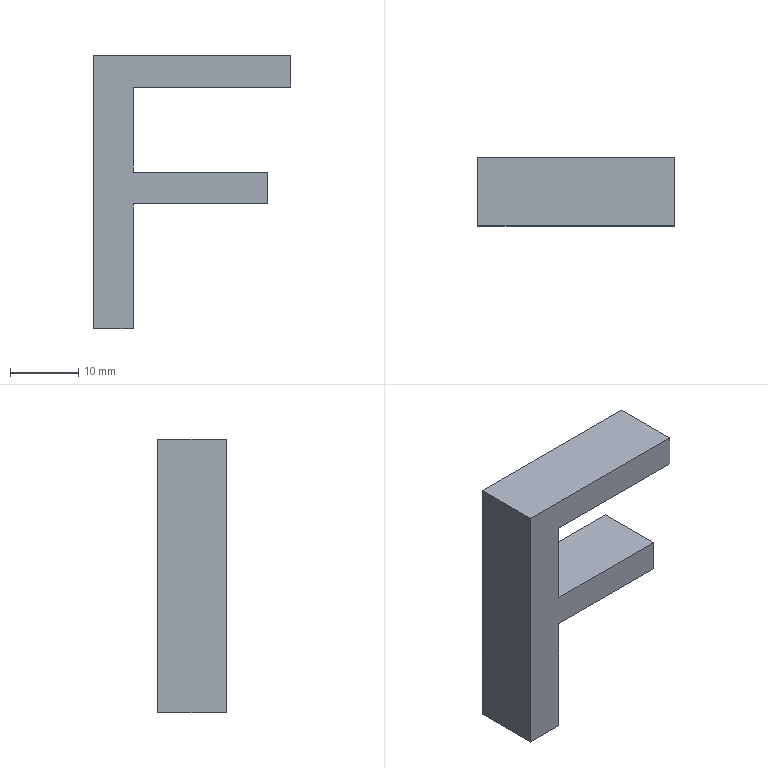Part | NX | features solid 2 | 1 solid | 12 faces | box 28.849 x 10 x 40 mm | volume 4328 mm3 | plane 12
STEP:
#1=CARTESIAN_POINT('',(-16.157,-1350.,-190.));
#2=VERTEX_POINT('',#1);
#3=CARTESIAN_POINT('',(-22.,-1350.,-190.));
#4=VERTEX_POINT('',#3);
#5=CARTESIAN_POINT('',(-16.157,-1350.,-190.));
#6=CARTESIAN_POINT('',(-18.105,-1350.,-190.));
#7=CARTESIAN_POINT('',(-20.052,-1350.,-190.));
#8=CARTESIAN_POINT('',(-22.,-1350.,-190.));
#9=B_SPLINE_CURVE_WITH_KNOTS('',3,(#5,#6,#7,#8),.UNSPECIFIED.,.F.,.F.,(4,4),(0.,0.03301),.PIECEWISE_BEZIER_KNOTS.);
#10=EDGE_CURVE('',#2,#4,#9,.T.);
#11=ORIENTED_EDGE('',*,*,#10,.F.);
#12=CARTESIAN_POINT('',(-16.157,-1360.,-190.));
#13=VERTEX_POINT('',#12);
#14=CARTESIAN_POINT('',(-16.157,-1360.,-190.));
#15=DIRECTION('',(0.,1.,0.));
#16=VECTOR('',#15,1000.);
#17=LINE('',#14,#16);
#18=EDGE_CURVE('',#13,#2,#17,.T.);
#19=ORIENTED_EDGE('',*,*,#18,.F.);
#20=CARTESIAN_POINT('',(-22.,-1360.,-190.));
#21=VERTEX_POINT('',#20);
#22=CARTESIAN_POINT('',(-16.157,-1360.,-190.));
#23=CARTESIAN_POINT('',(-18.105,-1360.,-190.));
#24=CARTESIAN_POINT('',(-20.052,-1360.,-190.));
#25=CARTESIAN_POINT('',(-22.,-1360.,-190.));
#26=B_SPLINE_CURVE_WITH_KNOTS('',3,(#22,#23,#24,#25),.UNSPECIFIED.,.F.,.F.,(4,4),(0.,0.03301),.PIECEWISE_BEZIER_KNOTS.);
#27=EDGE_CURVE('',#13,#21,#26,.T.);
#28=ORIENTED_EDGE('',*,*,#27,.T.);
#29=CARTESIAN_POINT('',(-22.,-1360.,-190.));
#30=DIRECTION('',(0.,1.,0.));
#31=VECTOR('',#30,1000.);
#32=LINE('',#29,#31);
#33=EDGE_CURVE('',#21,#4,#32,.T.);
#34=ORIENTED_EDGE('',*,*,#33,.T.);
#35=EDGE_LOOP('',(#11,#19,#28,#34));
#36=FACE_BOUND('',#35,.T.);
#37=CARTESIAN_POINT('',(-16.157,-1360.,-190.));
#38=DIRECTION('',(0.,0.,-1.));
#39=DIRECTION('',(0.,1.,0.));
#40=AXIS2_PLACEMENT_3D('',#37,#38,#39);
#41=PLANE('',#40);
#42=ADVANCED_FACE('',(#36),#41,.T.);
#43=CARTESIAN_POINT('',(-22.,-1350.,-150.));
#44=VERTEX_POINT('',#43);
#45=CARTESIAN_POINT('',(-22.,-1350.,-190.));
#46=CARTESIAN_POINT('',(-22.,-1350.,-176.667));
#47=CARTESIAN_POINT('',(-22.,-1350.,-163.333));
#48=CARTESIAN_POINT('',(-22.,-1350.,-150.));
#49=B_SPLINE_CURVE_WITH_KNOTS('',3,(#45,#46,#47,#48),.UNSPECIFIED.,.F.,.F.,(4,4),(0.03301,0.2589),.PIECEWISE_BEZIER_KNOTS.);
#50=EDGE_CURVE('',#4,#44,#49,.T.);
#51=ORIENTED_EDGE('',*,*,#50,.F.);
#52=ORIENTED_EDGE('',*,*,#33,.F.);
#53=CARTESIAN_POINT('',(-22.,-1360.,-150.));
#54=VERTEX_POINT('',#53);
#55=CARTESIAN_POINT('',(-22.,-1360.,-190.));
#56=CARTESIAN_POINT('',(-22.,-1360.,-176.667));
#57=CARTESIAN_POINT('',(-22.,-1360.,-163.333));
#58=CARTESIAN_POINT('',(-22.,-1360.,-150.));
#59=B_SPLINE_CURVE_WITH_KNOTS('',3,(#55,#56,#57,#58),.UNSPECIFIED.,.F.,.F.,(4,4),(0.03301,0.2589),.PIECEWISE_BEZIER_KNOTS.);
#60=EDGE_CURVE('',#21,#54,#59,.T.);
#61=ORIENTED_EDGE('',*,*,#60,.T.);
#62=CARTESIAN_POINT('',(-22.,-1360.,-150.));
#63=DIRECTION('',(0.,1.,0.));
#64=VECTOR('',#63,1000.);
#65=LINE('',#62,#64);
#66=EDGE_CURVE('',#54,#44,#65,.T.);
#67=ORIENTED_EDGE('',*,*,#66,.T.);
#68=EDGE_LOOP('',(#51,#52,#61,#67));
#69=FACE_BOUND('',#68,.T.);
#70=CARTESIAN_POINT('',(-22.,-1360.,-190.));
#71=DIRECTION('',(-1.,0.,0.));
#72=DIRECTION('',(0.,-1.,0.));
#73=AXIS2_PLACEMENT_3D('',#70,#71,#72);
#74=PLANE('',#73);
#75=ADVANCED_FACE('',(#69),#74,.T.);
#76=CARTESIAN_POINT('',(6.849,-1350.,-150.));
#77=VERTEX_POINT('',#76);
#78=CARTESIAN_POINT('',(-22.,-1350.,-150.));
#79=CARTESIAN_POINT('',(-12.384,-1350.,-150.));
#80=CARTESIAN_POINT('',(-2.767,-1350.,-150.));
#81=CARTESIAN_POINT('',(6.849,-1350.,-150.));
#82=B_SPLINE_CURVE_WITH_KNOTS('',3,(#78,#79,#80,#81),.UNSPECIFIED.,.F.,.F.,(4,4),(0.2589,0.4219),.PIECEWISE_BEZIER_KNOTS.);
#83=EDGE_CURVE('',#44,#77,#82,.T.);
#84=ORIENTED_EDGE('',*,*,#83,.F.);
#85=ORIENTED_EDGE('',*,*,#66,.F.);
#86=CARTESIAN_POINT('',(6.849,-1360.,-150.));
#87=VERTEX_POINT('',#86);
#88=CARTESIAN_POINT('',(-22.,-1360.,-150.));
#89=CARTESIAN_POINT('',(-12.384,-1360.,-150.));
#90=CARTESIAN_POINT('',(-2.767,-1360.,-150.));
#91=CARTESIAN_POINT('',(6.849,-1360.,-150.));
#92=B_SPLINE_CURVE_WITH_KNOTS('',3,(#88,#89,#90,#91),.UNSPECIFIED.,.F.,.F.,(4,4),(0.2589,0.4219),.PIECEWISE_BEZIER_KNOTS.);
#93=EDGE_CURVE('',#54,#87,#92,.T.);
#94=ORIENTED_EDGE('',*,*,#93,.T.);
#95=CARTESIAN_POINT('',(6.849,-1360.,-150.));
#96=DIRECTION('',(0.,1.,0.));
#97=VECTOR('',#96,1000.);
#98=LINE('',#95,#97);
#99=EDGE_CURVE('',#87,#77,#98,.T.);
#100=ORIENTED_EDGE('',*,*,#99,.T.);
#101=EDGE_LOOP('',(#84,#85,#94,#100));
#102=FACE_BOUND('',#101,.T.);
#103=CARTESIAN_POINT('',(-22.,-1360.,-150.));
#104=DIRECTION('',(0.,0.,1.));
#105=DIRECTION('',(0.,-1.,0.));
#106=AXIS2_PLACEMENT_3D('',#103,#104,#105);
#107=PLANE('',#106);
#108=ADVANCED_FACE('',(#102),#107,.T.);
#109=CARTESIAN_POINT('',(6.849,-1350.,-154.665));
#110=VERTEX_POINT('',#109);
#111=CARTESIAN_POINT('',(6.849,-1350.,-150.));
#112=CARTESIAN_POINT('',(6.849,-1350.,-151.555));
#113=CARTESIAN_POINT('',(6.849,-1350.,-153.11));
#114=CARTESIAN_POINT('',(6.849,-1350.,-154.665));
#115=B_SPLINE_CURVE_WITH_KNOTS('',3,(#111,#112,#113,#114),.UNSPECIFIED.,.F.,.F.,(4,4),(0.4219,0.4482),.PIECEWISE_BEZIER_KNOTS.);
#116=EDGE_CURVE('',#77,#110,#115,.T.);
#117=ORIENTED_EDGE('',*,*,#116,.F.);
#118=ORIENTED_EDGE('',*,*,#99,.F.);
#119=CARTESIAN_POINT('',(6.849,-1360.,-154.665));
#120=VERTEX_POINT('',#119);
#121=CARTESIAN_POINT('',(6.849,-1360.,-150.));
#122=CARTESIAN_POINT('',(6.849,-1360.,-151.555));
#123=CARTESIAN_POINT('',(6.849,-1360.,-153.11));
#124=CARTESIAN_POINT('',(6.849,-1360.,-154.665));
#125=B_SPLINE_CURVE_WITH_KNOTS('',3,(#121,#122,#123,#124),.UNSPECIFIED.,.F.,.F.,(4,4),(0.4219,0.4482),.PIECEWISE_BEZIER_KNOTS.);
#126=EDGE_CURVE('',#87,#120,#125,.T.);
#127=ORIENTED_EDGE('',*,*,#126,.T.);
#128=CARTESIAN_POINT('',(6.849,-1360.,-154.665));
#129=DIRECTION('',(0.,1.,0.));
#130=VECTOR('',#129,1000.);
#131=LINE('',#128,#130);
#132=EDGE_CURVE('',#120,#110,#131,.T.);
#133=ORIENTED_EDGE('',*,*,#132,.T.);
#134=EDGE_LOOP('',(#117,#118,#127,#133));
#135=FACE_BOUND('',#134,.T.);
#136=CARTESIAN_POINT('',(6.849,-1360.,-150.));
#137=DIRECTION('',(1.,0.,0.));
#138=DIRECTION('',(0.,1.,0.));
#139=AXIS2_PLACEMENT_3D('',#136,#137,#138);
#140=PLANE('',#139);
#141=ADVANCED_FACE('',(#135),#140,.T.);
#142=CARTESIAN_POINT('',(-16.157,-1350.,-154.665));
#143=VERTEX_POINT('',#142);
#144=CARTESIAN_POINT('',(6.849,-1350.,-154.665));
#145=CARTESIAN_POINT('',(-0.8196,-1350.,-154.665));
#146=CARTESIAN_POINT('',(-8.488,-1350.,-154.665));
#147=CARTESIAN_POINT('',(-16.157,-1350.,-154.665));
#148=B_SPLINE_CURVE_WITH_KNOTS('',3,(#144,#145,#146,#147),.UNSPECIFIED.,.F.,.F.,(4,4),(0.4482,0.5782),.PIECEWISE_BEZIER_KNOTS.);
#149=EDGE_CURVE('',#110,#143,#148,.T.);
#150=ORIENTED_EDGE('',*,*,#149,.F.);
#151=ORIENTED_EDGE('',*,*,#132,.F.);
#152=CARTESIAN_POINT('',(-16.157,-1360.,-154.665));
#153=VERTEX_POINT('',#152);
#154=CARTESIAN_POINT('',(6.849,-1360.,-154.665));
#155=CARTESIAN_POINT('',(-0.8196,-1360.,-154.665));
#156=CARTESIAN_POINT('',(-8.488,-1360.,-154.665));
#157=CARTESIAN_POINT('',(-16.157,-1360.,-154.665));
#158=B_SPLINE_CURVE_WITH_KNOTS('',3,(#154,#155,#156,#157),.UNSPECIFIED.,.F.,.F.,(4,4),(0.4482,0.5782),.PIECEWISE_BEZIER_KNOTS.);
#159=EDGE_CURVE('',#120,#153,#158,.T.);
#160=ORIENTED_EDGE('',*,*,#159,.T.);
#161=CARTESIAN_POINT('',(-16.157,-1360.,-154.665));
#162=DIRECTION('',(0.,1.,0.));
#163=VECTOR('',#162,1000.);
#164=LINE('',#161,#163);
#165=EDGE_CURVE('',#153,#143,#164,.T.);
#166=ORIENTED_EDGE('',*,*,#165,.T.);
#167=EDGE_LOOP('',(#150,#151,#160,#166));
#168=FACE_BOUND('',#167,.T.);
#169=CARTESIAN_POINT('',(6.849,-1360.,-154.665));
#170=DIRECTION('',(0.,0.,-1.));
#171=DIRECTION('',(0.,1.,0.));
#172=AXIS2_PLACEMENT_3D('',#169,#170,#171);
#173=PLANE('',#172);
#174=ADVANCED_FACE('',(#168),#173,.T.);
#175=CARTESIAN_POINT('',(-16.157,-1350.,-167.086));
#176=VERTEX_POINT('',#175);
#177=CARTESIAN_POINT('',(-16.157,-1350.,-154.665));
#178=CARTESIAN_POINT('',(-16.157,-1350.,-158.806));
#179=CARTESIAN_POINT('',(-16.157,-1350.,-162.946));
#180=CARTESIAN_POINT('',(-16.157,-1350.,-167.086));
#181=B_SPLINE_CURVE_WITH_KNOTS('',3,(#177,#178,#179,#180),.UNSPECIFIED.,.F.,.F.,(4,4),(0.5782,0.6483),.PIECEWISE_BEZIER_KNOTS.);
#182=EDGE_CURVE('',#143,#176,#181,.T.);
#183=ORIENTED_EDGE('',*,*,#182,.F.);
#184=ORIENTED_EDGE('',*,*,#165,.F.);
#185=CARTESIAN_POINT('',(-16.157,-1360.,-167.086));
#186=VERTEX_POINT('',#185);
#187=CARTESIAN_POINT('',(-16.157,-1360.,-154.665));
#188=CARTESIAN_POINT('',(-16.157,-1360.,-158.806));
#189=CARTESIAN_POINT('',(-16.157,-1360.,-162.946));
#190=CARTESIAN_POINT('',(-16.157,-1360.,-167.086));
#191=B_SPLINE_CURVE_WITH_KNOTS('',3,(#187,#188,#189,#190),.UNSPECIFIED.,.F.,.F.,(4,4),(0.5782,0.6483),.PIECEWISE_BEZIER_KNOTS.);
#192=EDGE_CURVE('',#153,#186,#191,.T.);
#193=ORIENTED_EDGE('',*,*,#192,.T.);
#194=CARTESIAN_POINT('',(-16.157,-1360.,-167.086));
#195=DIRECTION('',(0.,1.,0.));
#196=VECTOR('',#195,1000.);
#197=LINE('',#194,#196);
#198=EDGE_CURVE('',#186,#176,#197,.T.);
#199=ORIENTED_EDGE('',*,*,#198,.T.);
#200=EDGE_LOOP('',(#183,#184,#193,#199));
#201=FACE_BOUND('',#200,.T.);
#202=CARTESIAN_POINT('',(-16.157,-1360.,-154.665));
#203=DIRECTION('',(1.,0.,0.));
#204=DIRECTION('',(0.,1.,0.));
#205=AXIS2_PLACEMENT_3D('',#202,#203,#204);
#206=PLANE('',#205);
#207=ADVANCED_FACE('',(#201),#206,.T.);
#208=CARTESIAN_POINT('',(3.514,-1350.,-167.086));
#209=VERTEX_POINT('',#208);
#210=CARTESIAN_POINT('',(-16.157,-1350.,-167.086));
#211=CARTESIAN_POINT('',(-9.6,-1350.,-167.086));
#212=CARTESIAN_POINT('',(-3.043,-1350.,-167.086));
#213=CARTESIAN_POINT('',(3.514,-1350.,-167.086));
#214=B_SPLINE_CURVE_WITH_KNOTS('',3,(#210,#211,#212,#213),.UNSPECIFIED.,.F.,.F.,(4,4),(0.6483,0.7595),.PIECEWISE_BEZIER_KNOTS.);
#215=EDGE_CURVE('',#176,#209,#214,.T.);
#216=ORIENTED_EDGE('',*,*,#215,.F.);
#217=ORIENTED_EDGE('',*,*,#198,.F.);
#218=CARTESIAN_POINT('',(3.514,-1360.,-167.086));
#219=VERTEX_POINT('',#218);
#220=CARTESIAN_POINT('',(-16.157,-1360.,-167.086));
#221=CARTESIAN_POINT('',(-9.6,-1360.,-167.086));
#222=CARTESIAN_POINT('',(-3.043,-1360.,-167.086));
#223=CARTESIAN_POINT('',(3.514,-1360.,-167.086));
#224=B_SPLINE_CURVE_WITH_KNOTS('',3,(#220,#221,#222,#223),.UNSPECIFIED.,.F.,.F.,(4,4),(0.6483,0.7595),.PIECEWISE_BEZIER_KNOTS.);
#225=EDGE_CURVE('',#186,#219,#224,.T.);
#226=ORIENTED_EDGE('',*,*,#225,.T.);
#227=CARTESIAN_POINT('',(3.514,-1360.,-167.086));
#228=DIRECTION('',(0.,1.,0.));
#229=VECTOR('',#228,1000.);
#230=LINE('',#227,#229);
#231=EDGE_CURVE('',#219,#209,#230,.T.);
#232=ORIENTED_EDGE('',*,*,#231,.T.);
#233=EDGE_LOOP('',(#216,#217,#226,#232));
#234=FACE_BOUND('',#233,.T.);
#235=CARTESIAN_POINT('',(-16.157,-1360.,-167.086));
#236=DIRECTION('',(0.,0.,1.));
#237=DIRECTION('',(0.,-1.,0.));
#238=AXIS2_PLACEMENT_3D('',#235,#236,#237);
#239=PLANE('',#238);
#240=ADVANCED_FACE('',(#234),#239,.T.);
#241=CARTESIAN_POINT('',(3.514,-1350.,-171.751));
#242=VERTEX_POINT('',#241);
#243=CARTESIAN_POINT('',(3.514,-1350.,-167.086));
#244=CARTESIAN_POINT('',(3.514,-1350.,-168.641));
#245=CARTESIAN_POINT('',(3.514,-1350.,-170.196));
#246=CARTESIAN_POINT('',(3.514,-1350.,-171.751));
#247=B_SPLINE_CURVE_WITH_KNOTS('',3,(#243,#244,#245,#246),.UNSPECIFIED.,.F.,.F.,(4,4),(0.7595,0.7858),.PIECEWISE_BEZIER_KNOTS.);
#248=EDGE_CURVE('',#209,#242,#247,.T.);
#249=ORIENTED_EDGE('',*,*,#248,.F.);
#250=ORIENTED_EDGE('',*,*,#231,.F.);
#251=CARTESIAN_POINT('',(3.514,-1360.,-171.751));
#252=VERTEX_POINT('',#251);
#253=CARTESIAN_POINT('',(3.514,-1360.,-167.086));
#254=CARTESIAN_POINT('',(3.514,-1360.,-168.641));
#255=CARTESIAN_POINT('',(3.514,-1360.,-170.196));
#256=CARTESIAN_POINT('',(3.514,-1360.,-171.751));
#257=B_SPLINE_CURVE_WITH_KNOTS('',3,(#253,#254,#255,#256),.UNSPECIFIED.,.F.,.F.,(4,4),(0.7595,0.7858),.PIECEWISE_BEZIER_KNOTS.);
#258=EDGE_CURVE('',#219,#252,#257,.T.);
#259=ORIENTED_EDGE('',*,*,#258,.T.);
#260=CARTESIAN_POINT('',(3.514,-1360.,-171.751));
#261=DIRECTION('',(0.,1.,0.));
#262=VECTOR('',#261,1000.);
#263=LINE('',#260,#262);
#264=EDGE_CURVE('',#252,#242,#263,.T.);
#265=ORIENTED_EDGE('',*,*,#264,.T.);
#266=EDGE_LOOP('',(#249,#250,#259,#265));
#267=FACE_BOUND('',#266,.T.);
#268=CARTESIAN_POINT('',(3.514,-1360.,-167.086));
#269=DIRECTION('',(1.,0.,0.));
#270=DIRECTION('',(0.,1.,0.));
#271=AXIS2_PLACEMENT_3D('',#268,#269,#270);
#272=PLANE('',#271);
#273=ADVANCED_FACE('',(#267),#272,.T.);
#274=CARTESIAN_POINT('',(-16.157,-1350.,-171.751));
#275=VERTEX_POINT('',#274);
#276=CARTESIAN_POINT('',(3.514,-1350.,-171.751));
#277=CARTESIAN_POINT('',(-3.043,-1350.,-171.751));
#278=CARTESIAN_POINT('',(-9.6,-1350.,-171.751));
#279=CARTESIAN_POINT('',(-16.157,-1350.,-171.751));
#280=B_SPLINE_CURVE_WITH_KNOTS('',3,(#276,#277,#278,#279),.UNSPECIFIED.,.F.,.F.,(4,4),(0.7858,0.8969),.PIECEWISE_BEZIER_KNOTS.);
#281=EDGE_CURVE('',#242,#275,#280,.T.);
#282=ORIENTED_EDGE('',*,*,#281,.F.);
#283=ORIENTED_EDGE('',*,*,#264,.F.);
#284=CARTESIAN_POINT('',(-16.157,-1360.,-171.751));
#285=VERTEX_POINT('',#284);
#286=CARTESIAN_POINT('',(3.514,-1360.,-171.751));
#287=CARTESIAN_POINT('',(-3.043,-1360.,-171.751));
#288=CARTESIAN_POINT('',(-9.6,-1360.,-171.751));
#289=CARTESIAN_POINT('',(-16.157,-1360.,-171.751));
#290=B_SPLINE_CURVE_WITH_KNOTS('',3,(#286,#287,#288,#289),.UNSPECIFIED.,.F.,.F.,(4,4),(0.7858,0.8969),.PIECEWISE_BEZIER_KNOTS.);
#291=EDGE_CURVE('',#252,#285,#290,.T.);
#292=ORIENTED_EDGE('',*,*,#291,.T.);
#293=CARTESIAN_POINT('',(-16.157,-1360.,-171.751));
#294=DIRECTION('',(0.,1.,0.));
#295=VECTOR('',#294,1000.);
#296=LINE('',#293,#295);
#297=EDGE_CURVE('',#285,#275,#296,.T.);
#298=ORIENTED_EDGE('',*,*,#297,.T.);
#299=EDGE_LOOP('',(#282,#283,#292,#298));
#300=FACE_BOUND('',#299,.T.);
#301=CARTESIAN_POINT('',(3.514,-1360.,-171.751));
#302=DIRECTION('',(0.,0.,-1.));
#303=DIRECTION('',(0.,1.,0.));
#304=AXIS2_PLACEMENT_3D('',#301,#302,#303);
#305=PLANE('',#304);
#306=ADVANCED_FACE('',(#300),#305,.T.);
#307=CARTESIAN_POINT('',(-16.157,-1350.,-171.751));
#308=CARTESIAN_POINT('',(-16.157,-1350.,-177.834));
#309=CARTESIAN_POINT('',(-16.157,-1350.,-183.917));
#310=CARTESIAN_POINT('',(-16.157,-1350.,-190.));
#311=B_SPLINE_CURVE_WITH_KNOTS('',3,(#307,#308,#309,#310),.UNSPECIFIED.,.F.,.F.,(4,4),(0.8969,1.),.PIECEWISE_BEZIER_KNOTS.);
#312=EDGE_CURVE('',#275,#2,#311,.T.);
#313=ORIENTED_EDGE('',*,*,#312,.F.);
#314=ORIENTED_EDGE('',*,*,#297,.F.);
#315=CARTESIAN_POINT('',(-16.157,-1360.,-171.751));
#316=CARTESIAN_POINT('',(-16.157,-1360.,-177.834));
#317=CARTESIAN_POINT('',(-16.157,-1360.,-183.917));
#318=CARTESIAN_POINT('',(-16.157,-1360.,-190.));
#319=B_SPLINE_CURVE_WITH_KNOTS('',3,(#315,#316,#317,#318),.UNSPECIFIED.,.F.,.F.,(4,4),(0.8969,1.),.PIECEWISE_BEZIER_KNOTS.);
#320=EDGE_CURVE('',#285,#13,#319,.T.);
#321=ORIENTED_EDGE('',*,*,#320,.T.);
#322=ORIENTED_EDGE('',*,*,#18,.T.);
#323=EDGE_LOOP('',(#313,#314,#321,#322));
#324=FACE_BOUND('',#323,.T.);
#325=CARTESIAN_POINT('',(-16.157,-1360.,-171.751));
#326=DIRECTION('',(1.,0.,0.));
#327=DIRECTION('',(0.,1.,0.));
#328=AXIS2_PLACEMENT_3D('',#325,#326,#327);
#329=PLANE('',#328);
#330=ADVANCED_FACE('',(#324),#329,.T.);
#331=ORIENTED_EDGE('',*,*,#27,.F.);
#332=ORIENTED_EDGE('',*,*,#320,.F.);
#333=ORIENTED_EDGE('',*,*,#291,.F.);
#334=ORIENTED_EDGE('',*,*,#258,.F.);
#335=ORIENTED_EDGE('',*,*,#225,.F.);
#336=ORIENTED_EDGE('',*,*,#192,.F.);
#337=ORIENTED_EDGE('',*,*,#159,.F.);
#338=ORIENTED_EDGE('',*,*,#126,.F.);
#339=ORIENTED_EDGE('',*,*,#93,.F.);
#340=ORIENTED_EDGE('',*,*,#60,.F.);
#341=EDGE_LOOP('',(#331,#332,#333,#334,#335,#336,#337,#338,#339,#340));
#342=FACE_BOUND('',#341,.T.);
#343=CARTESIAN_POINT('',(-19.078,-1360.,-190.));
#344=DIRECTION('',(0.,-1.,0.));
#345=DIRECTION('',(1.,0.,0.));
#346=AXIS2_PLACEMENT_3D('',#343,#344,#345);
#347=PLANE('',#346);
#348=ADVANCED_FACE('',(#342),#347,.T.);
#349=ORIENTED_EDGE('',*,*,#10,.T.);
#350=ORIENTED_EDGE('',*,*,#50,.T.);
#351=ORIENTED_EDGE('',*,*,#83,.T.);
#352=ORIENTED_EDGE('',*,*,#116,.T.);
#353=ORIENTED_EDGE('',*,*,#149,.T.);
#354=ORIENTED_EDGE('',*,*,#182,.T.);
#355=ORIENTED_EDGE('',*,*,#215,.T.);
#356=ORIENTED_EDGE('',*,*,#248,.T.);
#357=ORIENTED_EDGE('',*,*,#281,.T.);
#358=ORIENTED_EDGE('',*,*,#312,.T.);
#359=EDGE_LOOP('',(#349,#350,#351,#352,#353,#354,#355,#356,#357,#358));
#360=FACE_BOUND('',#359,.T.);
#361=CARTESIAN_POINT('',(-19.078,-1350.,-190.));
#362=DIRECTION('',(0.,-1.,0.));
#363=DIRECTION('',(1.,0.,0.));
#364=AXIS2_PLACEMENT_3D('',#361,#362,#363);
#365=PLANE('',#364);
#366=ADVANCED_FACE('',(#360),#365,.F.);
#367=CLOSED_SHELL('',(#42,#75,#108,#141,#174,#207,#240,#273,#306,#330,#348,#366));
#368=MANIFOLD_SOLID_BREP('',#367);
#369=(LENGTH_UNIT()NAMED_UNIT(*)SI_UNIT(.MILLI.,.METRE.));
#370=UNCERTAINTY_MEASURE_WITH_UNIT(LENGTH_MEASURE(0.00001),#369,'','');
#371=(NAMED_UNIT(*)PLANE_ANGLE_UNIT()SI_UNIT($,.RADIAN.));
#372=(NAMED_UNIT(*)SI_UNIT($,.STERADIAN.)SOLID_ANGLE_UNIT());
#373=(GEOMETRIC_REPRESENTATION_CONTEXT(3)GLOBAL_UNCERTAINTY_ASSIGNED_CONTEXT((#370))GLOBAL_UNIT_ASSIGNED_CONTEXT((#369,#371,#372))REPRESENTATION_CONTEXT('',''));
#374=ADVANCED_BREP_SHAPE_REPRESENTATION('',(#368),#373);